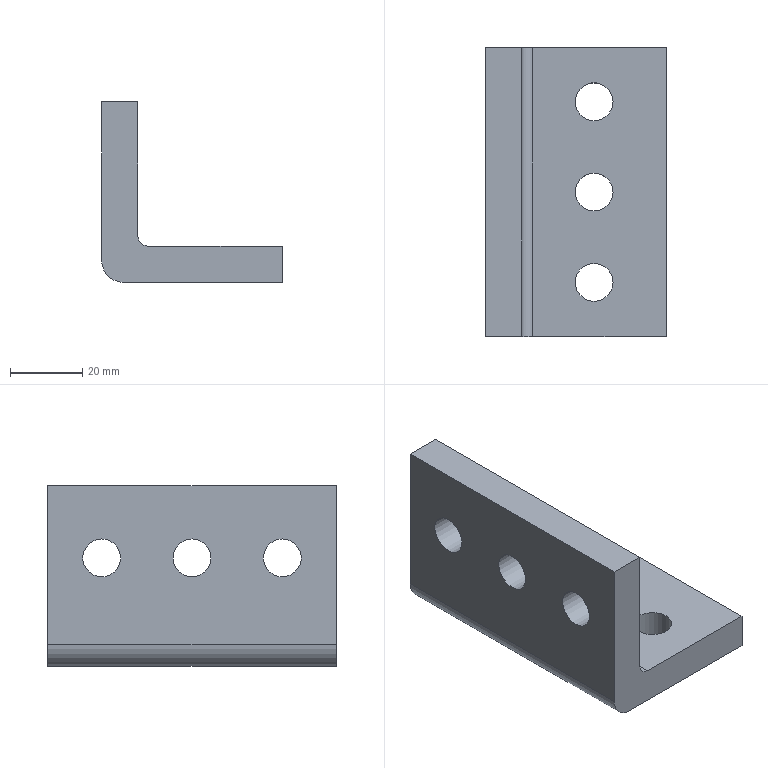Part | NX | features SIMPLE HOLE 6, DATUM_CSYS 4, SKETCH 3, BLEND 2, EXTRACT_DATUM_AXIS 2, EXTRACT_FACE 2, HOLE PACKAGE 2, EXTRUDE 1, Instance Feature 1, Mirror Feature 1 | 1 solid | 16 faces | box 50 x 80 x 50 mm | volume 66341 mm3 | plane 8 | cylinder 8 | commonest cylinder face diameters 10.5 x6 6 x1 12 x1
STEP:
#1=CARTESIAN_POINT('',(0.,25.,24.75));
#2=VERTEX_POINT('',#1);
#3=CARTESIAN_POINT('',(0.,25.,30.));
#4=DIRECTION('',(1.,0.,0.));
#5=DIRECTION('',(0.,0.,-1.));
#6=AXIS2_PLACEMENT_3D('',#3,#4,#5);
#7=CIRCLE('',#6,5.25);
#8=EDGE_CURVE('',#2,#2,#7,.T.);
#9=ORIENTED_EDGE('',*,*,#8,.T.);
#10=EDGE_LOOP('',(#9));
#11=FACE_BOUND('',#10,.T.);
#12=CARTESIAN_POINT('',(0.,0.,24.75));
#13=VERTEX_POINT('',#12);
#14=CARTESIAN_POINT('',(0.,0.,30.));
#15=DIRECTION('',(1.,0.,0.));
#16=DIRECTION('',(0.,0.,-1.));
#17=AXIS2_PLACEMENT_3D('',#14,#15,#16);
#18=CIRCLE('',#17,5.25);
#19=EDGE_CURVE('',#13,#13,#18,.T.);
#20=ORIENTED_EDGE('',*,*,#19,.T.);
#21=EDGE_LOOP('',(#20));
#22=FACE_BOUND('',#21,.T.);
#23=CARTESIAN_POINT('',(0.,-25.,24.75));
#24=VERTEX_POINT('',#23);
#25=CARTESIAN_POINT('',(0.,-25.,30.));
#26=DIRECTION('',(1.,0.,0.));
#27=DIRECTION('',(0.,0.,-1.));
#28=AXIS2_PLACEMENT_3D('',#25,#26,#27);
#29=CIRCLE('',#28,5.25);
#30=EDGE_CURVE('',#24,#24,#29,.T.);
#31=ORIENTED_EDGE('',*,*,#30,.T.);
#32=EDGE_LOOP('',(#31));
#33=FACE_BOUND('',#32,.T.);
#34=CARTESIAN_POINT('',(0.,40.,50.));
#35=VERTEX_POINT('',#34);
#36=CARTESIAN_POINT('',(0.,40.,6.));
#37=VERTEX_POINT('',#36);
#38=CARTESIAN_POINT('',(0.,40.,50.));
#39=DIRECTION('',(0.,0.,-1.));
#40=VECTOR('',#39,1000.);
#41=LINE('',#38,#40);
#42=EDGE_CURVE('',#35,#37,#41,.T.);
#43=ORIENTED_EDGE('',*,*,#42,.T.);
#44=CARTESIAN_POINT('',(0.,-40.,6.));
#45=VERTEX_POINT('',#44);
#46=CARTESIAN_POINT('',(0.,-40.,6.));
#47=DIRECTION('',(0.,1.,0.));
#48=VECTOR('',#47,1000.);
#49=LINE('',#46,#48);
#50=EDGE_CURVE('',#37,#45,#49,.F.);
#51=ORIENTED_EDGE('',*,*,#50,.T.);
#52=CARTESIAN_POINT('',(0.,-40.,50.));
#53=VERTEX_POINT('',#52);
#54=CARTESIAN_POINT('',(0.,-40.,50.));
#55=DIRECTION('',(0.,0.,-1.));
#56=VECTOR('',#55,1000.);
#57=LINE('',#54,#56);
#58=EDGE_CURVE('',#53,#45,#57,.T.);
#59=ORIENTED_EDGE('',*,*,#58,.F.);
#60=CARTESIAN_POINT('',(0.,-40.,50.));
#61=DIRECTION('',(0.,1.,0.));
#62=VECTOR('',#61,1000.);
#63=LINE('',#60,#62);
#64=EDGE_CURVE('',#53,#35,#63,.T.);
#65=ORIENTED_EDGE('',*,*,#64,.T.);
#66=EDGE_LOOP('',(#43,#51,#59,#65));
#67=FACE_BOUND('',#66,.T.);
#68=CARTESIAN_POINT('',(0.,-40.,50.));
#69=DIRECTION('',(1.,0.,0.));
#70=DIRECTION('',(0.,0.,-1.));
#71=AXIS2_PLACEMENT_3D('',#68,#69,#70);
#72=PLANE('',#71);
#73=ADVANCED_FACE('',(#11,#22,#33,#67),#72,.F.);
#74=CARTESIAN_POINT('',(35.25,25.,0.));
#75=VERTEX_POINT('',#74);
#76=CARTESIAN_POINT('',(30.,25.,0.));
#77=DIRECTION('',(0.,0.,1.));
#78=DIRECTION('',(1.,0.,0.));
#79=AXIS2_PLACEMENT_3D('',#76,#77,#78);
#80=CIRCLE('',#79,5.25);
#81=EDGE_CURVE('',#75,#75,#80,.T.);
#82=ORIENTED_EDGE('',*,*,#81,.T.);
#83=EDGE_LOOP('',(#82));
#84=FACE_BOUND('',#83,.T.);
#85=CARTESIAN_POINT('',(35.25,0.,0.));
#86=VERTEX_POINT('',#85);
#87=CARTESIAN_POINT('',(30.,0.,0.));
#88=DIRECTION('',(0.,0.,1.));
#89=DIRECTION('',(1.,0.,0.));
#90=AXIS2_PLACEMENT_3D('',#87,#88,#89);
#91=CIRCLE('',#90,5.25);
#92=EDGE_CURVE('',#86,#86,#91,.T.);
#93=ORIENTED_EDGE('',*,*,#92,.T.);
#94=EDGE_LOOP('',(#93));
#95=FACE_BOUND('',#94,.T.);
#96=CARTESIAN_POINT('',(35.25,-25.,0.));
#97=VERTEX_POINT('',#96);
#98=CARTESIAN_POINT('',(30.,-25.,0.));
#99=DIRECTION('',(0.,0.,1.));
#100=DIRECTION('',(1.,0.,0.));
#101=AXIS2_PLACEMENT_3D('',#98,#99,#100);
#102=CIRCLE('',#101,5.25);
#103=EDGE_CURVE('',#97,#97,#102,.T.);
#104=ORIENTED_EDGE('',*,*,#103,.T.);
#105=EDGE_LOOP('',(#104));
#106=FACE_BOUND('',#105,.T.);
#107=CARTESIAN_POINT('',(6.,-40.,0.));
#108=VERTEX_POINT('',#107);
#109=CARTESIAN_POINT('',(50.,-40.,0.));
#110=VERTEX_POINT('',#109);
#111=CARTESIAN_POINT('',(0.,-40.,0.));
#112=DIRECTION('',(1.,0.,0.));
#113=VECTOR('',#112,1000.);
#114=LINE('',#111,#113);
#115=EDGE_CURVE('',#108,#110,#114,.T.);
#116=ORIENTED_EDGE('',*,*,#115,.F.);
#117=CARTESIAN_POINT('',(6.,40.,0.));
#118=VERTEX_POINT('',#117);
#119=CARTESIAN_POINT('',(6.,-40.,0.));
#120=DIRECTION('',(0.,1.,0.));
#121=VECTOR('',#120,1000.);
#122=LINE('',#119,#121);
#123=EDGE_CURVE('',#108,#118,#122,.T.);
#124=ORIENTED_EDGE('',*,*,#123,.T.);
#125=CARTESIAN_POINT('',(50.,40.,0.));
#126=VERTEX_POINT('',#125);
#127=CARTESIAN_POINT('',(0.,40.,0.));
#128=DIRECTION('',(1.,0.,0.));
#129=VECTOR('',#128,1000.);
#130=LINE('',#127,#129);
#131=EDGE_CURVE('',#118,#126,#130,.T.);
#132=ORIENTED_EDGE('',*,*,#131,.T.);
#133=CARTESIAN_POINT('',(50.,-40.,0.));
#134=DIRECTION('',(0.,1.,0.));
#135=VECTOR('',#134,1000.);
#136=LINE('',#133,#135);
#137=EDGE_CURVE('',#110,#126,#136,.T.);
#138=ORIENTED_EDGE('',*,*,#137,.F.);
#139=EDGE_LOOP('',(#116,#124,#132,#138));
#140=FACE_BOUND('',#139,.T.);
#141=CARTESIAN_POINT('',(0.,-40.,0.));
#142=DIRECTION('',(0.,0.,1.));
#143=DIRECTION('',(1.,0.,0.));
#144=AXIS2_PLACEMENT_3D('',#141,#142,#143);
#145=PLANE('',#144);
#146=ADVANCED_FACE('',(#84,#95,#106,#140),#145,.F.);
#147=CARTESIAN_POINT('',(50.,40.,10.));
#148=VERTEX_POINT('',#147);
#149=CARTESIAN_POINT('',(50.,40.,0.));
#150=DIRECTION('',(0.,0.,1.));
#151=VECTOR('',#150,1000.);
#152=LINE('',#149,#151);
#153=EDGE_CURVE('',#126,#148,#152,.T.);
#154=ORIENTED_EDGE('',*,*,#153,.T.);
#155=CARTESIAN_POINT('',(50.,-40.,10.));
#156=VERTEX_POINT('',#155);
#157=CARTESIAN_POINT('',(50.,-40.,10.));
#158=DIRECTION('',(0.,1.,0.));
#159=VECTOR('',#158,1000.);
#160=LINE('',#157,#159);
#161=EDGE_CURVE('',#156,#148,#160,.T.);
#162=ORIENTED_EDGE('',*,*,#161,.F.);
#163=CARTESIAN_POINT('',(50.,-40.,0.));
#164=DIRECTION('',(0.,0.,1.));
#165=VECTOR('',#164,1000.);
#166=LINE('',#163,#165);
#167=EDGE_CURVE('',#110,#156,#166,.T.);
#168=ORIENTED_EDGE('',*,*,#167,.F.);
#169=ORIENTED_EDGE('',*,*,#137,.T.);
#170=EDGE_LOOP('',(#154,#162,#168,#169));
#171=FACE_BOUND('',#170,.T.);
#172=CARTESIAN_POINT('',(50.,-40.,0.));
#173=DIRECTION('',(-1.,0.,0.));
#174=DIRECTION('',(0.,0.,1.));
#175=AXIS2_PLACEMENT_3D('',#172,#173,#174);
#176=PLANE('',#175);
#177=ADVANCED_FACE('',(#171),#176,.F.);
#178=CARTESIAN_POINT('',(24.75,25.,10.));
#179=VERTEX_POINT('',#178);
#180=CARTESIAN_POINT('',(30.,25.,10.));
#181=DIRECTION('',(0.,0.,-1.));
#182=DIRECTION('',(-1.,0.,0.));
#183=AXIS2_PLACEMENT_3D('',#180,#181,#182);
#184=CIRCLE('',#183,5.25);
#185=EDGE_CURVE('',#179,#179,#184,.T.);
#186=ORIENTED_EDGE('',*,*,#185,.T.);
#187=EDGE_LOOP('',(#186));
#188=FACE_BOUND('',#187,.T.);
#189=CARTESIAN_POINT('',(24.75,0.,10.));
#190=VERTEX_POINT('',#189);
#191=CARTESIAN_POINT('',(30.,0.,10.));
#192=DIRECTION('',(0.,0.,-1.));
#193=DIRECTION('',(-1.,0.,0.));
#194=AXIS2_PLACEMENT_3D('',#191,#192,#193);
#195=CIRCLE('',#194,5.25);
#196=EDGE_CURVE('',#190,#190,#195,.T.);
#197=ORIENTED_EDGE('',*,*,#196,.T.);
#198=EDGE_LOOP('',(#197));
#199=FACE_BOUND('',#198,.T.);
#200=CARTESIAN_POINT('',(24.75,-25.,10.));
#201=VERTEX_POINT('',#200);
#202=CARTESIAN_POINT('',(30.,-25.,10.));
#203=DIRECTION('',(0.,0.,-1.));
#204=DIRECTION('',(-1.,0.,0.));
#205=AXIS2_PLACEMENT_3D('',#202,#203,#204);
#206=CIRCLE('',#205,5.25);
#207=EDGE_CURVE('',#201,#201,#206,.T.);
#208=ORIENTED_EDGE('',*,*,#207,.T.);
#209=EDGE_LOOP('',(#208));
#210=FACE_BOUND('',#209,.T.);
#211=CARTESIAN_POINT('',(13.,40.,10.));
#212=VERTEX_POINT('',#211);
#213=CARTESIAN_POINT('',(50.,40.,10.));
#214=DIRECTION('',(-1.,0.,0.));
#215=VECTOR('',#214,1000.);
#216=LINE('',#213,#215);
#217=EDGE_CURVE('',#148,#212,#216,.T.);
#218=ORIENTED_EDGE('',*,*,#217,.T.);
#219=CARTESIAN_POINT('',(13.,-40.,10.));
#220=VERTEX_POINT('',#219);
#221=CARTESIAN_POINT('',(13.,-40.,10.));
#222=DIRECTION('',(0.,1.,0.));
#223=VECTOR('',#222,1000.);
#224=LINE('',#221,#223);
#225=EDGE_CURVE('',#212,#220,#224,.F.);
#226=ORIENTED_EDGE('',*,*,#225,.T.);
#227=CARTESIAN_POINT('',(50.,-40.,10.));
#228=DIRECTION('',(-1.,0.,0.));
#229=VECTOR('',#228,1000.);
#230=LINE('',#227,#229);
#231=EDGE_CURVE('',#156,#220,#230,.T.);
#232=ORIENTED_EDGE('',*,*,#231,.F.);
#233=ORIENTED_EDGE('',*,*,#161,.T.);
#234=EDGE_LOOP('',(#218,#226,#232,#233));
#235=FACE_BOUND('',#234,.T.);
#236=CARTESIAN_POINT('',(50.,-40.,10.));
#237=DIRECTION('',(0.,0.,-1.));
#238=DIRECTION('',(-1.,0.,0.));
#239=AXIS2_PLACEMENT_3D('',#236,#237,#238);
#240=PLANE('',#239);
#241=ADVANCED_FACE('',(#188,#199,#210,#235),#240,.F.);
#242=CARTESIAN_POINT('',(10.,25.,35.25));
#243=VERTEX_POINT('',#242);
#244=CARTESIAN_POINT('',(10.,25.,30.));
#245=DIRECTION('',(-1.,0.,0.));
#246=DIRECTION('',(0.,0.,1.));
#247=AXIS2_PLACEMENT_3D('',#244,#245,#246);
#248=CIRCLE('',#247,5.25);
#249=EDGE_CURVE('',#243,#243,#248,.T.);
#250=ORIENTED_EDGE('',*,*,#249,.T.);
#251=EDGE_LOOP('',(#250));
#252=FACE_BOUND('',#251,.T.);
#253=CARTESIAN_POINT('',(10.,0.,35.25));
#254=VERTEX_POINT('',#253);
#255=CARTESIAN_POINT('',(10.,0.,30.));
#256=DIRECTION('',(-1.,0.,0.));
#257=DIRECTION('',(0.,0.,1.));
#258=AXIS2_PLACEMENT_3D('',#255,#256,#257);
#259=CIRCLE('',#258,5.25);
#260=EDGE_CURVE('',#254,#254,#259,.T.);
#261=ORIENTED_EDGE('',*,*,#260,.T.);
#262=EDGE_LOOP('',(#261));
#263=FACE_BOUND('',#262,.T.);
#264=CARTESIAN_POINT('',(10.,-25.,35.25));
#265=VERTEX_POINT('',#264);
#266=CARTESIAN_POINT('',(10.,-25.,30.));
#267=DIRECTION('',(-1.,0.,0.));
#268=DIRECTION('',(0.,0.,1.));
#269=AXIS2_PLACEMENT_3D('',#266,#267,#268);
#270=CIRCLE('',#269,5.25);
#271=EDGE_CURVE('',#265,#265,#270,.T.);
#272=ORIENTED_EDGE('',*,*,#271,.T.);
#273=EDGE_LOOP('',(#272));
#274=FACE_BOUND('',#273,.T.);
#275=CARTESIAN_POINT('',(10.,-40.,13.));
#276=VERTEX_POINT('',#275);
#277=CARTESIAN_POINT('',(10.,-40.,50.));
#278=VERTEX_POINT('',#277);
#279=CARTESIAN_POINT('',(10.,-40.,10.));
#280=DIRECTION('',(0.,0.,1.));
#281=VECTOR('',#280,1000.);
#282=LINE('',#279,#281);
#283=EDGE_CURVE('',#276,#278,#282,.T.);
#284=ORIENTED_EDGE('',*,*,#283,.F.);
#285=CARTESIAN_POINT('',(10.,40.,13.));
#286=VERTEX_POINT('',#285);
#287=CARTESIAN_POINT('',(10.,40.,13.));
#288=DIRECTION('',(0.,1.,0.));
#289=VECTOR('',#288,1000.);
#290=LINE('',#287,#289);
#291=EDGE_CURVE('',#276,#286,#290,.T.);
#292=ORIENTED_EDGE('',*,*,#291,.T.);
#293=CARTESIAN_POINT('',(10.,40.,50.));
#294=VERTEX_POINT('',#293);
#295=CARTESIAN_POINT('',(10.,40.,10.));
#296=DIRECTION('',(0.,0.,1.));
#297=VECTOR('',#296,1000.);
#298=LINE('',#295,#297);
#299=EDGE_CURVE('',#286,#294,#298,.T.);
#300=ORIENTED_EDGE('',*,*,#299,.T.);
#301=CARTESIAN_POINT('',(10.,-40.,50.));
#302=DIRECTION('',(0.,1.,0.));
#303=VECTOR('',#302,1000.);
#304=LINE('',#301,#303);
#305=EDGE_CURVE('',#278,#294,#304,.T.);
#306=ORIENTED_EDGE('',*,*,#305,.F.);
#307=EDGE_LOOP('',(#284,#292,#300,#306));
#308=FACE_BOUND('',#307,.T.);
#309=CARTESIAN_POINT('',(10.,-40.,10.));
#310=DIRECTION('',(-1.,0.,0.));
#311=DIRECTION('',(0.,0.,1.));
#312=AXIS2_PLACEMENT_3D('',#309,#310,#311);
#313=PLANE('',#312);
#314=ADVANCED_FACE('',(#252,#263,#274,#308),#313,.F.);
#315=CARTESIAN_POINT('',(10.,40.,50.));
#316=DIRECTION('',(-1.,0.,0.));
#317=VECTOR('',#316,1000.);
#318=LINE('',#315,#317);
#319=EDGE_CURVE('',#294,#35,#318,.T.);
#320=ORIENTED_EDGE('',*,*,#319,.T.);
#321=ORIENTED_EDGE('',*,*,#64,.F.);
#322=CARTESIAN_POINT('',(10.,-40.,50.));
#323=DIRECTION('',(-1.,0.,0.));
#324=VECTOR('',#323,1000.);
#325=LINE('',#322,#324);
#326=EDGE_CURVE('',#278,#53,#325,.T.);
#327=ORIENTED_EDGE('',*,*,#326,.F.);
#328=ORIENTED_EDGE('',*,*,#305,.T.);
#329=EDGE_LOOP('',(#320,#321,#327,#328));
#330=FACE_BOUND('',#329,.T.);
#331=CARTESIAN_POINT('',(10.,-40.,50.));
#332=DIRECTION('',(0.,0.,-1.));
#333=DIRECTION('',(-1.,0.,0.));
#334=AXIS2_PLACEMENT_3D('',#331,#332,#333);
#335=PLANE('',#334);
#336=ADVANCED_FACE('',(#330),#335,.F.);
#337=ORIENTED_EDGE('',*,*,#58,.T.);
#338=CARTESIAN_POINT('',(6.,-40.,6.));
#339=DIRECTION('',(0.,-1.,0.));
#340=DIRECTION('',(0.,0.,-1.));
#341=AXIS2_PLACEMENT_3D('',#338,#339,#340);
#342=CIRCLE('',#341,6.);
#343=EDGE_CURVE('',#45,#108,#342,.T.);
#344=ORIENTED_EDGE('',*,*,#343,.T.);
#345=ORIENTED_EDGE('',*,*,#115,.T.);
#346=ORIENTED_EDGE('',*,*,#167,.T.);
#347=ORIENTED_EDGE('',*,*,#231,.T.);
#348=CARTESIAN_POINT('',(13.,-40.,13.));
#349=DIRECTION('',(0.,-1.,0.));
#350=DIRECTION('',(0.,0.,-1.));
#351=AXIS2_PLACEMENT_3D('',#348,#349,#350);
#352=CIRCLE('',#351,3.);
#353=EDGE_CURVE('',#220,#276,#352,.F.);
#354=ORIENTED_EDGE('',*,*,#353,.T.);
#355=ORIENTED_EDGE('',*,*,#283,.T.);
#356=ORIENTED_EDGE('',*,*,#326,.T.);
#357=EDGE_LOOP('',(#337,#344,#345,#346,#347,#354,#355,#356));
#358=FACE_BOUND('',#357,.T.);
#359=CARTESIAN_POINT('',(0.,-40.,0.));
#360=DIRECTION('',(0.,-1.,0.));
#361=DIRECTION('',(0.,0.,-1.));
#362=AXIS2_PLACEMENT_3D('',#359,#360,#361);
#363=PLANE('',#362);
#364=ADVANCED_FACE('',(#358),#363,.T.);
#365=ORIENTED_EDGE('',*,*,#131,.F.);
#366=CARTESIAN_POINT('',(6.,40.,6.));
#367=DIRECTION('',(0.,-1.,0.));
#368=DIRECTION('',(0.,0.,-1.));
#369=AXIS2_PLACEMENT_3D('',#366,#367,#368);
#370=CIRCLE('',#369,6.);
#371=EDGE_CURVE('',#118,#37,#370,.F.);
#372=ORIENTED_EDGE('',*,*,#371,.T.);
#373=ORIENTED_EDGE('',*,*,#42,.F.);
#374=ORIENTED_EDGE('',*,*,#319,.F.);
#375=ORIENTED_EDGE('',*,*,#299,.F.);
#376=CARTESIAN_POINT('',(13.,40.,13.));
#377=DIRECTION('',(0.,-1.,0.));
#378=DIRECTION('',(0.,0.,-1.));
#379=AXIS2_PLACEMENT_3D('',#376,#377,#378);
#380=CIRCLE('',#379,3.);
#381=EDGE_CURVE('',#286,#212,#380,.T.);
#382=ORIENTED_EDGE('',*,*,#381,.T.);
#383=ORIENTED_EDGE('',*,*,#217,.F.);
#384=ORIENTED_EDGE('',*,*,#153,.F.);
#385=EDGE_LOOP('',(#365,#372,#373,#374,#375,#382,#383,#384));
#386=FACE_BOUND('',#385,.T.);
#387=CARTESIAN_POINT('',(0.,40.,0.));
#388=DIRECTION('',(0.,-1.,0.));
#389=DIRECTION('',(0.,0.,-1.));
#390=AXIS2_PLACEMENT_3D('',#387,#388,#389);
#391=PLANE('',#390);
#392=ADVANCED_FACE('',(#386),#391,.F.);
#393=ORIENTED_EDGE('',*,*,#271,.F.);
#394=EDGE_LOOP('',(#393));
#395=FACE_BOUND('',#394,.T.);
#396=ORIENTED_EDGE('',*,*,#30,.F.);
#397=EDGE_LOOP('',(#396));
#398=FACE_BOUND('',#397,.T.);
#399=CARTESIAN_POINT('',(10.,-25.,30.));
#400=DIRECTION('',(-1.,0.,0.));
#401=DIRECTION('',(0.,0.,1.));
#402=AXIS2_PLACEMENT_3D('',#399,#400,#401);
#403=CYLINDRICAL_SURFACE('',#402,5.25);
#404=ADVANCED_FACE('',(#395,#398),#403,.F.);
#405=ORIENTED_EDGE('',*,*,#260,.F.);
#406=EDGE_LOOP('',(#405));
#407=FACE_BOUND('',#406,.T.);
#408=ORIENTED_EDGE('',*,*,#19,.F.);
#409=EDGE_LOOP('',(#408));
#410=FACE_BOUND('',#409,.T.);
#411=CARTESIAN_POINT('',(10.,0.,30.));
#412=DIRECTION('',(-1.,0.,0.));
#413=DIRECTION('',(0.,0.,1.));
#414=AXIS2_PLACEMENT_3D('',#411,#412,#413);
#415=CYLINDRICAL_SURFACE('',#414,5.25);
#416=ADVANCED_FACE('',(#407,#410),#415,.F.);
#417=ORIENTED_EDGE('',*,*,#249,.F.);
#418=EDGE_LOOP('',(#417));
#419=FACE_BOUND('',#418,.T.);
#420=ORIENTED_EDGE('',*,*,#8,.F.);
#421=EDGE_LOOP('',(#420));
#422=FACE_BOUND('',#421,.T.);
#423=CARTESIAN_POINT('',(10.,25.,30.));
#424=DIRECTION('',(-1.,0.,0.));
#425=DIRECTION('',(0.,0.,1.));
#426=AXIS2_PLACEMENT_3D('',#423,#424,#425);
#427=CYLINDRICAL_SURFACE('',#426,5.25);
#428=ADVANCED_FACE('',(#419,#422),#427,.F.);
#429=ORIENTED_EDGE('',*,*,#207,.F.);
#430=EDGE_LOOP('',(#429));
#431=FACE_BOUND('',#430,.T.);
#432=ORIENTED_EDGE('',*,*,#103,.F.);
#433=EDGE_LOOP('',(#432));
#434=FACE_BOUND('',#433,.T.);
#435=CARTESIAN_POINT('',(30.,-25.,10.));
#436=DIRECTION('',(0.,0.,-1.));
#437=DIRECTION('',(-1.,0.,0.));
#438=AXIS2_PLACEMENT_3D('',#435,#436,#437);
#439=CYLINDRICAL_SURFACE('',#438,5.25);
#440=ADVANCED_FACE('',(#431,#434),#439,.F.);
#441=ORIENTED_EDGE('',*,*,#196,.F.);
#442=EDGE_LOOP('',(#441));
#443=FACE_BOUND('',#442,.T.);
#444=ORIENTED_EDGE('',*,*,#92,.F.);
#445=EDGE_LOOP('',(#444));
#446=FACE_BOUND('',#445,.T.);
#447=CARTESIAN_POINT('',(30.,0.,10.));
#448=DIRECTION('',(0.,0.,-1.));
#449=DIRECTION('',(-1.,0.,0.));
#450=AXIS2_PLACEMENT_3D('',#447,#448,#449);
#451=CYLINDRICAL_SURFACE('',#450,5.25);
#452=ADVANCED_FACE('',(#443,#446),#451,.F.);
#453=ORIENTED_EDGE('',*,*,#185,.F.);
#454=EDGE_LOOP('',(#453));
#455=FACE_BOUND('',#454,.T.);
#456=ORIENTED_EDGE('',*,*,#81,.F.);
#457=EDGE_LOOP('',(#456));
#458=FACE_BOUND('',#457,.T.);
#459=CARTESIAN_POINT('',(30.,25.,10.));
#460=DIRECTION('',(0.,0.,-1.));
#461=DIRECTION('',(-1.,0.,0.));
#462=AXIS2_PLACEMENT_3D('',#459,#460,#461);
#463=CYLINDRICAL_SURFACE('',#462,5.25);
#464=ADVANCED_FACE('',(#455,#458),#463,.F.);
#465=ORIENTED_EDGE('',*,*,#353,.F.);
#466=ORIENTED_EDGE('',*,*,#225,.F.);
#467=ORIENTED_EDGE('',*,*,#381,.F.);
#468=ORIENTED_EDGE('',*,*,#291,.F.);
#469=EDGE_LOOP('',(#465,#466,#467,#468));
#470=FACE_BOUND('',#469,.T.);
#471=CARTESIAN_POINT('',(13.,-40.,13.));
#472=DIRECTION('',(0.,-1.,0.));
#473=DIRECTION('',(0.,0.,-1.));
#474=AXIS2_PLACEMENT_3D('',#471,#472,#473);
#475=CYLINDRICAL_SURFACE('',#474,3.);
#476=ADVANCED_FACE('',(#470),#475,.F.);
#477=ORIENTED_EDGE('',*,*,#343,.F.);
#478=ORIENTED_EDGE('',*,*,#50,.F.);
#479=ORIENTED_EDGE('',*,*,#371,.F.);
#480=ORIENTED_EDGE('',*,*,#123,.F.);
#481=EDGE_LOOP('',(#477,#478,#479,#480));
#482=FACE_BOUND('',#481,.T.);
#483=CARTESIAN_POINT('',(6.,-40.,6.));
#484=DIRECTION('',(0.,1.,0.));
#485=DIRECTION('',(0.,0.,1.));
#486=AXIS2_PLACEMENT_3D('',#483,#484,#485);
#487=CYLINDRICAL_SURFACE('',#486,6.);
#488=ADVANCED_FACE('',(#482),#487,.T.);
#489=CLOSED_SHELL('',(#73,#146,#177,#241,#314,#336,#364,#392,#404,#416,#428,#440,#452,#464,#476,#488));
#490=MANIFOLD_SOLID_BREP('',#489);
#491=(LENGTH_UNIT()NAMED_UNIT(*)SI_UNIT(.MILLI.,.METRE.));
#492=UNCERTAINTY_MEASURE_WITH_UNIT(LENGTH_MEASURE(0.00001),#491,'','');
#493=(NAMED_UNIT(*)PLANE_ANGLE_UNIT()SI_UNIT($,.RADIAN.));
#494=(NAMED_UNIT(*)SI_UNIT($,.STERADIAN.)SOLID_ANGLE_UNIT());
#495=(GEOMETRIC_REPRESENTATION_CONTEXT(3)GLOBAL_UNCERTAINTY_ASSIGNED_CONTEXT((#492))GLOBAL_UNIT_ASSIGNED_CONTEXT((#491,#493,#494))REPRESENTATION_CONTEXT('',''));
#496=ADVANCED_BREP_SHAPE_REPRESENTATION('',(#490),#495);